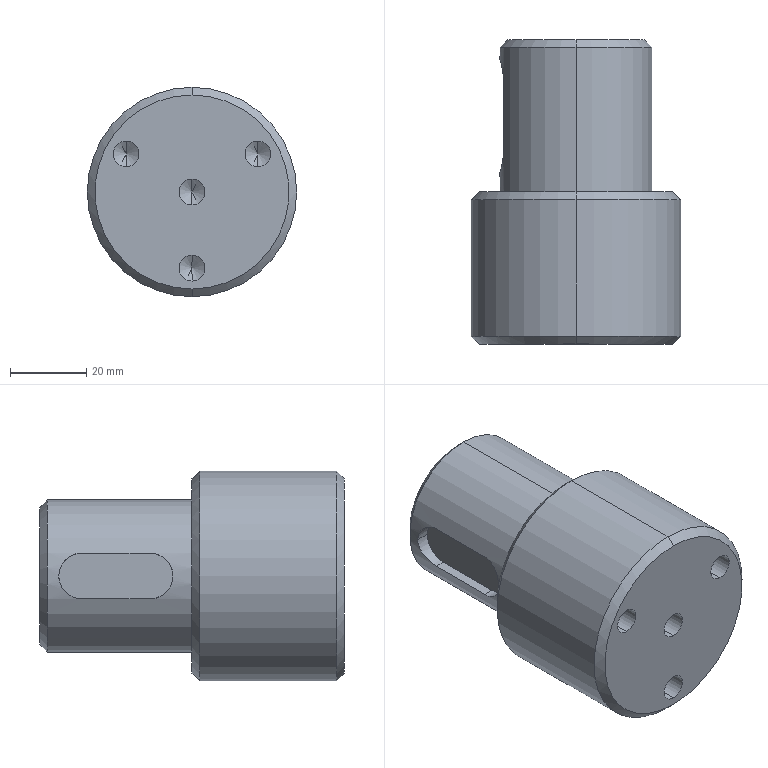Part | SolidWorks | features HoleWzd 2, Chamfer 1, Fillet 1, ICE 1, Revolution 1 | 1 solid | 40 faces | box 55 x 80 x 55 mm | volume 132055 mm3 | cylinder 18 | cone 16 | plane 6 | commonest cylinder face diameters 6.8 x8 12 x4 15.5 x2 40 x2 55 x2
STEP:
#1=CARTESIAN_POINT('',(0.,22.25,-16.6));
#2=VERTEX_POINT('',#1);
#3=CARTESIAN_POINT('',(0.,22.25,-23.4));
#4=VERTEX_POINT('',#3);
#5=CARTESIAN_POINT('',(0.,22.25,-20.));
#6=DIRECTION('',(0.,-1.,0.));
#7=DIRECTION('',(0.,0.,-1.));
#8=AXIS2_PLACEMENT_3D('',#5,#6,#7);
#9=CIRCLE('',#8,3.4);
#10=EDGE_CURVE('',#2,#4,#9,.T.);
#11=ORIENTED_EDGE('',*,*,#10,.F.);
#12=CARTESIAN_POINT('',(0.,0.,-16.6));
#13=VERTEX_POINT('',#12);
#14=CARTESIAN_POINT('',(0.,0.,-16.6));
#15=DIRECTION('',(0.,-1.,0.));
#16=VECTOR('',#15,1000.);
#17=LINE('',#14,#16);
#18=EDGE_CURVE('',#2,#13,#17,.T.);
#19=ORIENTED_EDGE('',*,*,#18,.T.);
#20=CARTESIAN_POINT('',(0.,0.,-23.4));
#21=VERTEX_POINT('',#20);
#22=CARTESIAN_POINT('',(0.,0.,-20.));
#23=DIRECTION('',(0.,-1.,0.));
#24=DIRECTION('',(0.,0.,-1.));
#25=AXIS2_PLACEMENT_3D('',#22,#23,#24);
#26=CIRCLE('',#25,3.4);
#27=EDGE_CURVE('',#13,#21,#26,.T.);
#28=ORIENTED_EDGE('',*,*,#27,.T.);
#29=CARTESIAN_POINT('',(0.,0.,-23.4));
#30=DIRECTION('',(0.,-1.,0.));
#31=VECTOR('',#30,1000.);
#32=LINE('',#29,#31);
#33=EDGE_CURVE('',#4,#21,#32,.T.);
#34=ORIENTED_EDGE('',*,*,#33,.F.);
#35=EDGE_LOOP('',(#11,#19,#28,#34));
#36=FACE_OUTER_BOUND('',#35,.T.);
#37=CARTESIAN_POINT('',(0.,0.,-20.));
#38=DIRECTION('',(0.,-1.,0.));
#39=DIRECTION('',(0.,0.,-1.));
#40=AXIS2_PLACEMENT_3D('',#37,#38,#39);
#41=CYLINDRICAL_SURFACE('',#40,3.4);
#42=ADVANCED_FACE('',(#36),#41,.F.);
#43=CARTESIAN_POINT('',(0.,24.293,-20.));
#44=VERTEX_POINT('',#43);
#45=CARTESIAN_POINT('',(0.,22.25,-23.4));
#46=DIRECTION('',(0.,-0.515,-0.8572));
#47=VECTOR('',#46,1000.);
#48=LINE('',#45,#47);
#49=EDGE_CURVE('',#44,#4,#48,.T.);
#50=ORIENTED_EDGE('',*,*,#49,.F.);
#51=CARTESIAN_POINT('',(0.,22.25,-16.6));
#52=DIRECTION('',(0.,-0.515,0.8572));
#53=VECTOR('',#52,1000.);
#54=LINE('',#51,#53);
#55=EDGE_CURVE('',#44,#2,#54,.T.);
#56=ORIENTED_EDGE('',*,*,#55,.T.);
#57=ORIENTED_EDGE('',*,*,#10,.T.);
#58=EDGE_LOOP('',(#50,#56,#57));
#59=FACE_OUTER_BOUND('',#58,.T.);
#60=CARTESIAN_POINT('',(0.,22.25,-20.));
#61=DIRECTION('',(0.,-1.,0.));
#62=DIRECTION('',(0.,0.,-1.));
#63=AXIS2_PLACEMENT_3D('',#60,#61,#62);
#64=CONICAL_SURFACE('',#63,3.4,1.03);
#65=ADVANCED_FACE('',(#59),#64,.F.);
#66=CARTESIAN_POINT('',(-17.321,22.25,13.4));
#67=VERTEX_POINT('',#66);
#68=CARTESIAN_POINT('',(-17.321,22.25,6.6));
#69=VERTEX_POINT('',#68);
#70=CARTESIAN_POINT('',(-17.321,22.25,10.));
#71=DIRECTION('',(0.,-1.,0.));
#72=DIRECTION('',(0.,0.,-1.));
#73=AXIS2_PLACEMENT_3D('',#70,#71,#72);
#74=CIRCLE('',#73,3.4);
#75=EDGE_CURVE('',#67,#69,#74,.T.);
#76=ORIENTED_EDGE('',*,*,#75,.F.);
#77=CARTESIAN_POINT('',(-17.321,0.,13.4));
#78=VERTEX_POINT('',#77);
#79=CARTESIAN_POINT('',(-17.321,0.,13.4));
#80=DIRECTION('',(0.,-1.,0.));
#81=VECTOR('',#80,1000.);
#82=LINE('',#79,#81);
#83=EDGE_CURVE('',#67,#78,#82,.T.);
#84=ORIENTED_EDGE('',*,*,#83,.T.);
#85=CARTESIAN_POINT('',(-17.321,0.,6.6));
#86=VERTEX_POINT('',#85);
#87=CARTESIAN_POINT('',(-17.321,0.,10.));
#88=DIRECTION('',(0.,-1.,0.));
#89=DIRECTION('',(0.,0.,-1.));
#90=AXIS2_PLACEMENT_3D('',#87,#88,#89);
#91=CIRCLE('',#90,3.4);
#92=EDGE_CURVE('',#78,#86,#91,.T.);
#93=ORIENTED_EDGE('',*,*,#92,.T.);
#94=CARTESIAN_POINT('',(-17.321,0.,6.6));
#95=DIRECTION('',(0.,-1.,0.));
#96=VECTOR('',#95,1000.);
#97=LINE('',#94,#96);
#98=EDGE_CURVE('',#69,#86,#97,.T.);
#99=ORIENTED_EDGE('',*,*,#98,.F.);
#100=EDGE_LOOP('',(#76,#84,#93,#99));
#101=FACE_OUTER_BOUND('',#100,.T.);
#102=CARTESIAN_POINT('',(-17.321,0.,10.));
#103=DIRECTION('',(0.,-1.,0.));
#104=DIRECTION('',(0.,0.,-1.));
#105=AXIS2_PLACEMENT_3D('',#102,#103,#104);
#106=CYLINDRICAL_SURFACE('',#105,3.4);
#107=ADVANCED_FACE('',(#101),#106,.F.);
#108=CARTESIAN_POINT('',(-17.321,24.293,10.));
#109=VERTEX_POINT('',#108);
#110=CARTESIAN_POINT('',(-17.321,22.25,6.6));
#111=DIRECTION('',(0.,-0.515,-0.8572));
#112=VECTOR('',#111,1000.);
#113=LINE('',#110,#112);
#114=EDGE_CURVE('',#109,#69,#113,.T.);
#115=ORIENTED_EDGE('',*,*,#114,.F.);
#116=CARTESIAN_POINT('',(-17.321,22.25,13.4));
#117=DIRECTION('',(0.,-0.515,0.8572));
#118=VECTOR('',#117,1000.);
#119=LINE('',#116,#118);
#120=EDGE_CURVE('',#109,#67,#119,.T.);
#121=ORIENTED_EDGE('',*,*,#120,.T.);
#122=ORIENTED_EDGE('',*,*,#75,.T.);
#123=EDGE_LOOP('',(#115,#121,#122));
#124=FACE_OUTER_BOUND('',#123,.T.);
#125=CARTESIAN_POINT('',(-17.321,22.25,10.));
#126=DIRECTION('',(0.,-1.,0.));
#127=DIRECTION('',(0.,0.,-1.));
#128=AXIS2_PLACEMENT_3D('',#125,#126,#127);
#129=CONICAL_SURFACE('',#128,3.4,1.03);
#130=ADVANCED_FACE('',(#124),#129,.F.);
#131=CARTESIAN_POINT('',(17.321,22.25,13.4));
#132=VERTEX_POINT('',#131);
#133=CARTESIAN_POINT('',(17.321,22.25,6.6));
#134=VERTEX_POINT('',#133);
#135=CARTESIAN_POINT('',(17.321,22.25,10.));
#136=DIRECTION('',(0.,-1.,0.));
#137=DIRECTION('',(0.,0.,-1.));
#138=AXIS2_PLACEMENT_3D('',#135,#136,#137);
#139=CIRCLE('',#138,3.4);
#140=EDGE_CURVE('',#132,#134,#139,.T.);
#141=ORIENTED_EDGE('',*,*,#140,.F.);
#142=CARTESIAN_POINT('',(17.321,0.,13.4));
#143=VERTEX_POINT('',#142);
#144=CARTESIAN_POINT('',(17.321,0.,13.4));
#145=DIRECTION('',(0.,-1.,0.));
#146=VECTOR('',#145,1000.);
#147=LINE('',#144,#146);
#148=EDGE_CURVE('',#132,#143,#147,.T.);
#149=ORIENTED_EDGE('',*,*,#148,.T.);
#150=CARTESIAN_POINT('',(17.321,0.,6.6));
#151=VERTEX_POINT('',#150);
#152=CARTESIAN_POINT('',(17.321,0.,10.));
#153=DIRECTION('',(0.,-1.,0.));
#154=DIRECTION('',(0.,0.,-1.));
#155=AXIS2_PLACEMENT_3D('',#152,#153,#154);
#156=CIRCLE('',#155,3.4);
#157=EDGE_CURVE('',#143,#151,#156,.T.);
#158=ORIENTED_EDGE('',*,*,#157,.T.);
#159=CARTESIAN_POINT('',(17.321,0.,6.6));
#160=DIRECTION('',(0.,-1.,0.));
#161=VECTOR('',#160,1000.);
#162=LINE('',#159,#161);
#163=EDGE_CURVE('',#134,#151,#162,.T.);
#164=ORIENTED_EDGE('',*,*,#163,.F.);
#165=EDGE_LOOP('',(#141,#149,#158,#164));
#166=FACE_OUTER_BOUND('',#165,.T.);
#167=CARTESIAN_POINT('',(17.321,0.,10.));
#168=DIRECTION('',(0.,-1.,0.));
#169=DIRECTION('',(0.,0.,-1.));
#170=AXIS2_PLACEMENT_3D('',#167,#168,#169);
#171=CYLINDRICAL_SURFACE('',#170,3.4);
#172=ADVANCED_FACE('',(#166),#171,.F.);
#173=CARTESIAN_POINT('',(17.321,24.293,10.));
#174=VERTEX_POINT('',#173);
#175=CARTESIAN_POINT('',(17.321,22.25,6.6));
#176=DIRECTION('',(0.,-0.515,-0.8572));
#177=VECTOR('',#176,1000.);
#178=LINE('',#175,#177);
#179=EDGE_CURVE('',#174,#134,#178,.T.);
#180=ORIENTED_EDGE('',*,*,#179,.F.);
#181=CARTESIAN_POINT('',(17.321,22.25,13.4));
#182=DIRECTION('',(0.,-0.515,0.8572));
#183=VECTOR('',#182,1000.);
#184=LINE('',#181,#183);
#185=EDGE_CURVE('',#174,#132,#184,.T.);
#186=ORIENTED_EDGE('',*,*,#185,.T.);
#187=ORIENTED_EDGE('',*,*,#140,.T.);
#188=EDGE_LOOP('',(#180,#186,#187));
#189=FACE_OUTER_BOUND('',#188,.T.);
#190=CARTESIAN_POINT('',(17.321,22.25,10.));
#191=DIRECTION('',(0.,-1.,0.));
#192=DIRECTION('',(0.,0.,-1.));
#193=AXIS2_PLACEMENT_3D('',#190,#191,#192);
#194=CONICAL_SURFACE('',#193,3.4,1.03);
#195=ADVANCED_FACE('',(#189),#194,.F.);
#196=CARTESIAN_POINT('',(0.,22.25,3.4));
#197=VERTEX_POINT('',#196);
#198=CARTESIAN_POINT('',(0.,22.25,-3.4));
#199=VERTEX_POINT('',#198);
#200=CARTESIAN_POINT('',(0.,22.25,0.));
#201=DIRECTION('',(0.,-1.,0.));
#202=DIRECTION('',(0.,0.,-1.));
#203=AXIS2_PLACEMENT_3D('',#200,#201,#202);
#204=CIRCLE('',#203,3.4);
#205=EDGE_CURVE('',#197,#199,#204,.T.);
#206=ORIENTED_EDGE('',*,*,#205,.F.);
#207=CARTESIAN_POINT('',(0.,0.,3.4));
#208=VERTEX_POINT('',#207);
#209=CARTESIAN_POINT('',(0.,0.,3.4));
#210=DIRECTION('',(0.,-1.,0.));
#211=VECTOR('',#210,1000.);
#212=LINE('',#209,#211);
#213=EDGE_CURVE('',#197,#208,#212,.T.);
#214=ORIENTED_EDGE('',*,*,#213,.T.);
#215=CARTESIAN_POINT('',(0.,0.,-3.4));
#216=VERTEX_POINT('',#215);
#217=CARTESIAN_POINT('',(0.,0.,0.));
#218=DIRECTION('',(0.,-1.,0.));
#219=DIRECTION('',(0.,0.,-1.));
#220=AXIS2_PLACEMENT_3D('',#217,#218,#219);
#221=CIRCLE('',#220,3.4);
#222=EDGE_CURVE('',#208,#216,#221,.T.);
#223=ORIENTED_EDGE('',*,*,#222,.T.);
#224=CARTESIAN_POINT('',(0.,0.,-3.4));
#225=DIRECTION('',(0.,-1.,0.));
#226=VECTOR('',#225,1000.);
#227=LINE('',#224,#226);
#228=EDGE_CURVE('',#199,#216,#227,.T.);
#229=ORIENTED_EDGE('',*,*,#228,.F.);
#230=EDGE_LOOP('',(#206,#214,#223,#229));
#231=FACE_OUTER_BOUND('',#230,.T.);
#232=CARTESIAN_POINT('',(0.,0.,0.));
#233=DIRECTION('',(0.,-1.,0.));
#234=DIRECTION('',(0.,0.,-1.));
#235=AXIS2_PLACEMENT_3D('',#232,#233,#234);
#236=CYLINDRICAL_SURFACE('',#235,3.4);
#237=ADVANCED_FACE('',(#231),#236,.F.);
#238=CARTESIAN_POINT('',(0.,24.293,0.));
#239=VERTEX_POINT('',#238);
#240=CARTESIAN_POINT('',(0.,22.25,-3.4));
#241=DIRECTION('',(0.,-0.515,-0.8572));
#242=VECTOR('',#241,1000.);
#243=LINE('',#240,#242);
#244=EDGE_CURVE('',#239,#199,#243,.T.);
#245=ORIENTED_EDGE('',*,*,#244,.F.);
#246=CARTESIAN_POINT('',(0.,22.25,3.4));
#247=DIRECTION('',(0.,-0.515,0.8572));
#248=VECTOR('',#247,1000.);
#249=LINE('',#246,#248);
#250=EDGE_CURVE('',#239,#197,#249,.T.);
#251=ORIENTED_EDGE('',*,*,#250,.T.);
#252=ORIENTED_EDGE('',*,*,#205,.T.);
#253=EDGE_LOOP('',(#245,#251,#252));
#254=FACE_OUTER_BOUND('',#253,.T.);
#255=CARTESIAN_POINT('',(0.,22.25,0.));
#256=DIRECTION('',(0.,-1.,0.));
#257=DIRECTION('',(0.,0.,-1.));
#258=AXIS2_PLACEMENT_3D('',#255,#256,#257);
#259=CONICAL_SURFACE('',#258,3.4,1.03);
#260=ADVANCED_FACE('',(#254),#259,.F.);
#261=CARTESIAN_POINT('',(0.,80.,18.));
#262=VERTEX_POINT('',#261);
#263=CARTESIAN_POINT('',(0.,80.,-18.));
#264=VERTEX_POINT('',#263);
#265=CARTESIAN_POINT('',(0.,80.,0.));
#266=DIRECTION('',(0.,1.,0.));
#267=DIRECTION('',(0.,0.,1.));
#268=AXIS2_PLACEMENT_3D('',#265,#266,#267);
#269=CIRCLE('',#268,18.);
#270=EDGE_CURVE('',#262,#264,#269,.T.);
#271=ORIENTED_EDGE('',*,*,#270,.F.);
#272=CARTESIAN_POINT('',(0.,78.,20.));
#273=VERTEX_POINT('',#272);
#274=CARTESIAN_POINT('',(0.,78.,20.));
#275=DIRECTION('',(0.,-0.7071,0.7071));
#276=VECTOR('',#275,1000.);
#277=LINE('',#274,#276);
#278=EDGE_CURVE('',#262,#273,#277,.T.);
#279=ORIENTED_EDGE('',*,*,#278,.T.);
#280=CARTESIAN_POINT('',(0.,78.,-20.));
#281=VERTEX_POINT('',#280);
#282=CARTESIAN_POINT('',(0.,78.,0.));
#283=DIRECTION('',(0.,-1.,0.));
#284=DIRECTION('',(0.,0.,1.));
#285=AXIS2_PLACEMENT_3D('',#282,#283,#284);
#286=CIRCLE('',#285,20.);
#287=EDGE_CURVE('',#281,#273,#286,.T.);
#288=ORIENTED_EDGE('',*,*,#287,.F.);
#289=CARTESIAN_POINT('',(0.,78.,-20.));
#290=DIRECTION('',(0.,-0.7071,-0.7071));
#291=VECTOR('',#290,1000.);
#292=LINE('',#289,#291);
#293=EDGE_CURVE('',#264,#281,#292,.T.);
#294=ORIENTED_EDGE('',*,*,#293,.F.);
#295=EDGE_LOOP('',(#271,#279,#288,#294));
#296=FACE_OUTER_BOUND('',#295,.T.);
#297=CARTESIAN_POINT('',(0.,78.,0.));
#298=DIRECTION('',(0.,-1.,0.));
#299=DIRECTION('',(0.,0.,-1.));
#300=AXIS2_PLACEMENT_3D('',#297,#298,#299);
#301=CONICAL_SURFACE('',#300,20.,0.7854);
#302=ADVANCED_FACE('',(#296),#301,.T.);
#303=CARTESIAN_POINT('',(0.,40.,25.5));
#304=VERTEX_POINT('',#303);
#305=CARTESIAN_POINT('',(0.,40.,-25.5));
#306=VERTEX_POINT('',#305);
#307=CARTESIAN_POINT('',(0.,40.,0.));
#308=DIRECTION('',(0.,1.,0.));
#309=DIRECTION('',(0.,0.,1.));
#310=AXIS2_PLACEMENT_3D('',#307,#308,#309);
#311=CIRCLE('',#310,25.5);
#312=EDGE_CURVE('',#304,#306,#311,.T.);
#313=ORIENTED_EDGE('',*,*,#312,.F.);
#314=CARTESIAN_POINT('',(0.,38.,27.5));
#315=VERTEX_POINT('',#314);
#316=CARTESIAN_POINT('',(0.,38.,27.5));
#317=DIRECTION('',(0.,-0.7071,0.7071));
#318=VECTOR('',#317,1000.);
#319=LINE('',#316,#318);
#320=EDGE_CURVE('',#304,#315,#319,.T.);
#321=ORIENTED_EDGE('',*,*,#320,.T.);
#322=CARTESIAN_POINT('',(0.,38.,-27.5));
#323=VERTEX_POINT('',#322);
#324=CARTESIAN_POINT('',(0.,38.,0.));
#325=DIRECTION('',(0.,-1.,0.));
#326=DIRECTION('',(0.,0.,1.));
#327=AXIS2_PLACEMENT_3D('',#324,#325,#326);
#328=CIRCLE('',#327,27.5);
#329=EDGE_CURVE('',#323,#315,#328,.T.);
#330=ORIENTED_EDGE('',*,*,#329,.F.);
#331=CARTESIAN_POINT('',(0.,38.,-27.5));
#332=DIRECTION('',(0.,-0.7071,-0.7071));
#333=VECTOR('',#332,1000.);
#334=LINE('',#331,#333);
#335=EDGE_CURVE('',#306,#323,#334,.T.);
#336=ORIENTED_EDGE('',*,*,#335,.F.);
#337=EDGE_LOOP('',(#313,#321,#330,#336));
#338=FACE_OUTER_BOUND('',#337,.T.);
#339=CARTESIAN_POINT('',(0.,38.,0.));
#340=DIRECTION('',(0.,-1.,0.));
#341=DIRECTION('',(0.,0.,-1.));
#342=AXIS2_PLACEMENT_3D('',#339,#340,#341);
#343=CONICAL_SURFACE('',#342,27.5,0.7854);
#344=ADVANCED_FACE('',(#338),#343,.T.);
#345=CARTESIAN_POINT('',(0.,0.,-25.5));
#346=VERTEX_POINT('',#345);
#347=CARTESIAN_POINT('',(0.,0.,25.5));
#348=VERTEX_POINT('',#347);
#349=CARTESIAN_POINT('',(0.,0.,0.));
#350=DIRECTION('',(0.,-1.,0.));
#351=DIRECTION('',(0.,0.,-1.));
#352=AXIS2_PLACEMENT_3D('',#349,#350,#351);
#353=CIRCLE('',#352,25.5);
#354=EDGE_CURVE('',#346,#348,#353,.T.);
#355=ORIENTED_EDGE('',*,*,#354,.F.);
#356=CARTESIAN_POINT('',(0.,2.,-27.5));
#357=VERTEX_POINT('',#356);
#358=CARTESIAN_POINT('',(0.,0.,-25.5));
#359=DIRECTION('',(0.,0.7071,-0.7071));
#360=VECTOR('',#359,1000.);
#361=LINE('',#358,#360);
#362=EDGE_CURVE('',#346,#357,#361,.T.);
#363=ORIENTED_EDGE('',*,*,#362,.T.);
#364=CARTESIAN_POINT('',(0.,2.,27.5));
#365=VERTEX_POINT('',#364);
#366=CARTESIAN_POINT('',(0.,2.,0.));
#367=DIRECTION('',(0.,1.,0.));
#368=DIRECTION('',(0.,0.,-1.));
#369=AXIS2_PLACEMENT_3D('',#366,#367,#368);
#370=CIRCLE('',#369,27.5);
#371=EDGE_CURVE('',#365,#357,#370,.T.);
#372=ORIENTED_EDGE('',*,*,#371,.F.);
#373=CARTESIAN_POINT('',(0.,0.,25.5));
#374=DIRECTION('',(0.,0.7071,0.7071));
#375=VECTOR('',#374,1000.);
#376=LINE('',#373,#375);
#377=EDGE_CURVE('',#348,#365,#376,.T.);
#378=ORIENTED_EDGE('',*,*,#377,.F.);
#379=EDGE_LOOP('',(#355,#363,#372,#378));
#380=FACE_OUTER_BOUND('',#379,.T.);
#381=CARTESIAN_POINT('',(0.,0.,0.));
#382=DIRECTION('',(0.,1.,0.));
#383=DIRECTION('',(0.,0.,1.));
#384=AXIS2_PLACEMENT_3D('',#381,#382,#383);
#385=CONICAL_SURFACE('',#384,25.5,0.7854);
#386=ADVANCED_FACE('',(#380),#385,.T.);
#387=CARTESIAN_POINT('',(0.,39.5,-7.75));
#388=VERTEX_POINT('',#387);
#389=CARTESIAN_POINT('',(0.,39.5,7.75));
#390=VERTEX_POINT('',#389);
#391=CARTESIAN_POINT('',(0.,39.5,0.));
#392=DIRECTION('',(0.,1.,0.));
#393=DIRECTION('',(0.,0.,1.));
#394=AXIS2_PLACEMENT_3D('',#391,#392,#393);
#395=CIRCLE('',#394,7.75);
#396=EDGE_CURVE('',#388,#390,#395,.T.);
#397=ORIENTED_EDGE('',*,*,#396,.F.);
#398=CARTESIAN_POINT('',(0.,80.,-7.75));
#399=VERTEX_POINT('',#398);
#400=CARTESIAN_POINT('',(0.,80.,-7.75));
#401=DIRECTION('',(0.,1.,0.));
#402=VECTOR('',#401,1000.);
#403=LINE('',#400,#402);
#404=EDGE_CURVE('',#388,#399,#403,.T.);
#405=ORIENTED_EDGE('',*,*,#404,.T.);
#406=CARTESIAN_POINT('',(0.,80.,7.75));
#407=VERTEX_POINT('',#406);
#408=CARTESIAN_POINT('',(0.,80.,0.));
#409=DIRECTION('',(0.,1.,0.));
#410=DIRECTION('',(0.,0.,1.));
#411=AXIS2_PLACEMENT_3D('',#408,#409,#410);
#412=CIRCLE('',#411,7.75);
#413=EDGE_CURVE('',#399,#407,#412,.T.);
#414=ORIENTED_EDGE('',*,*,#413,.T.);
#415=CARTESIAN_POINT('',(0.,80.,7.75));
#416=DIRECTION('',(0.,1.,0.));
#417=VECTOR('',#416,1000.);
#418=LINE('',#415,#417);
#419=EDGE_CURVE('',#390,#407,#418,.T.);
#420=ORIENTED_EDGE('',*,*,#419,.F.);
#421=EDGE_LOOP('',(#397,#405,#414,#420));
#422=FACE_OUTER_BOUND('',#421,.T.);
#423=CARTESIAN_POINT('',(0.,80.,0.));
#424=DIRECTION('',(0.,1.,0.));
#425=DIRECTION('',(0.,0.,1.));
#426=AXIS2_PLACEMENT_3D('',#423,#424,#425);
#427=CYLINDRICAL_SURFACE('',#426,7.75);
#428=ADVANCED_FACE('',(#422),#427,.F.);
#429=CARTESIAN_POINT('',(0.,34.843,0.));
#430=VERTEX_POINT('',#429);
#431=CARTESIAN_POINT('',(0.,39.5,7.75));
#432=DIRECTION('',(0.,0.515,0.8572));
#433=VECTOR('',#432,1000.);
#434=LINE('',#431,#433);
#435=EDGE_CURVE('',#430,#390,#434,.T.);
#436=ORIENTED_EDGE('',*,*,#435,.F.);
#437=CARTESIAN_POINT('',(0.,39.5,-7.75));
#438=DIRECTION('',(0.,0.515,-0.8572));
#439=VECTOR('',#438,1000.);
#440=LINE('',#437,#439);
#441=EDGE_CURVE('',#430,#388,#440,.T.);
#442=ORIENTED_EDGE('',*,*,#441,.T.);
#443=ORIENTED_EDGE('',*,*,#396,.T.);
#444=EDGE_LOOP('',(#436,#442,#443));
#445=FACE_OUTER_BOUND('',#444,.T.);
#446=CARTESIAN_POINT('',(0.,39.5,0.));
#447=DIRECTION('',(0.,1.,0.));
#448=DIRECTION('',(0.,0.,1.));
#449=AXIS2_PLACEMENT_3D('',#446,#447,#448);
#450=CONICAL_SURFACE('',#449,7.75,1.03);
#451=ADVANCED_FACE('',(#445),#450,.F.);
#452=ORIENTED_EDGE('',*,*,#329,.T.);
#453=CARTESIAN_POINT('',(0.,0.,27.5));
#454=DIRECTION('',(0.,-1.,0.));
#455=VECTOR('',#454,1000.);
#456=LINE('',#453,#455);
#457=EDGE_CURVE('',#315,#365,#456,.T.);
#458=ORIENTED_EDGE('',*,*,#457,.T.);
#459=ORIENTED_EDGE('',*,*,#371,.T.);
#460=CARTESIAN_POINT('',(0.,0.,-27.5));
#461=DIRECTION('',(0.,-1.,0.));
#462=VECTOR('',#461,1000.);
#463=LINE('',#460,#462);
#464=EDGE_CURVE('',#323,#357,#463,.T.);
#465=ORIENTED_EDGE('',*,*,#464,.F.);
#466=EDGE_LOOP('',(#452,#458,#459,#465));
#467=FACE_OUTER_BOUND('',#466,.T.);
#468=CARTESIAN_POINT('',(0.,0.,0.));
#469=DIRECTION('',(0.,-1.,0.));
#470=DIRECTION('',(0.,0.,-1.));
#471=AXIS2_PLACEMENT_3D('',#468,#469,#470);
#472=CYLINDRICAL_SURFACE('',#471,27.5);
#473=ADVANCED_FACE('',(#467),#472,.T.);
#474=ORIENTED_EDGE('',*,*,#287,.T.);
#475=CARTESIAN_POINT('',(0.,40.,20.));
#476=VERTEX_POINT('',#475);
#477=CARTESIAN_POINT('',(0.,0.,20.));
#478=DIRECTION('',(0.,-1.,0.));
#479=VECTOR('',#478,1000.);
#480=LINE('',#477,#479);
#481=EDGE_CURVE('',#273,#476,#480,.T.);
#482=ORIENTED_EDGE('',*,*,#481,.T.);
#483=CARTESIAN_POINT('',(0.,40.,-20.));
#484=VERTEX_POINT('',#483);
#485=CARTESIAN_POINT('',(0.,40.,0.));
#486=DIRECTION('',(0.,-1.,0.));
#487=DIRECTION('',(0.,0.,-1.));
#488=AXIS2_PLACEMENT_3D('',#485,#486,#487);
#489=CIRCLE('',#488,20.);
#490=EDGE_CURVE('',#484,#476,#489,.T.);
#491=ORIENTED_EDGE('',*,*,#490,.F.);
#492=CARTESIAN_POINT('',(0.,0.,-20.));
#493=DIRECTION('',(0.,-1.,0.));
#494=VECTOR('',#493,1000.);
#495=LINE('',#492,#494);
#496=EDGE_CURVE('',#281,#484,#495,.T.);
#497=ORIENTED_EDGE('',*,*,#496,.F.);
#498=EDGE_LOOP('',(#474,#482,#491,#497));
#499=FACE_OUTER_BOUND('',#498,.T.);
#500=CARTESIAN_POINT('',(0.,0.,0.));
#501=DIRECTION('',(0.,-1.,0.));
#502=DIRECTION('',(0.,0.,-1.));
#503=AXIS2_PLACEMENT_3D('',#500,#501,#502);
#504=CYLINDRICAL_SURFACE('',#503,20.);
#505=ADVANCED_FACE('',(#499),#504,.T.);
#506=CARTESIAN_POINT('',(0.,0.,-20.));
#507=DIRECTION('',(0.,-1.,0.));
#508=DIRECTION('',(0.,0.,-1.));
#509=AXIS2_PLACEMENT_3D('',#506,#507,#508);
#510=CIRCLE('',#509,3.4);
#511=EDGE_CURVE('',#21,#13,#510,.T.);
#512=ORIENTED_EDGE('',*,*,#511,.F.);
#513=ORIENTED_EDGE('',*,*,#27,.F.);
#514=EDGE_LOOP('',(#512,#513));
#515=FACE_BOUND('',#514,.T.);
#516=CARTESIAN_POINT('',(-17.321,0.,10.));
#517=DIRECTION('',(0.,-1.,0.));
#518=DIRECTION('',(0.,0.,-1.));
#519=AXIS2_PLACEMENT_3D('',#516,#517,#518);
#520=CIRCLE('',#519,3.4);
#521=EDGE_CURVE('',#86,#78,#520,.T.);
#522=ORIENTED_EDGE('',*,*,#521,.F.);
#523=ORIENTED_EDGE('',*,*,#92,.F.);
#524=EDGE_LOOP('',(#522,#523));
#525=FACE_BOUND('',#524,.T.);
#526=CARTESIAN_POINT('',(17.321,0.,10.));
#527=DIRECTION('',(0.,-1.,0.));
#528=DIRECTION('',(0.,0.,-1.));
#529=AXIS2_PLACEMENT_3D('',#526,#527,#528);
#530=CIRCLE('',#529,3.4);
#531=EDGE_CURVE('',#151,#143,#530,.T.);
#532=ORIENTED_EDGE('',*,*,#531,.F.);
#533=ORIENTED_EDGE('',*,*,#157,.F.);
#534=EDGE_LOOP('',(#532,#533));
#535=FACE_BOUND('',#534,.T.);
#536=CARTESIAN_POINT('',(0.,0.,0.));
#537=DIRECTION('',(0.,-1.,0.));
#538=DIRECTION('',(0.,0.,-1.));
#539=AXIS2_PLACEMENT_3D('',#536,#537,#538);
#540=CIRCLE('',#539,3.4);
#541=EDGE_CURVE('',#216,#208,#540,.T.);
#542=ORIENTED_EDGE('',*,*,#541,.F.);
#543=ORIENTED_EDGE('',*,*,#222,.F.);
#544=EDGE_LOOP('',(#542,#543));
#545=FACE_BOUND('',#544,.T.);
#546=CARTESIAN_POINT('',(0.,0.,0.));
#547=DIRECTION('',(0.,-1.,0.));
#548=DIRECTION('',(0.,0.,-1.));
#549=AXIS2_PLACEMENT_3D('',#546,#547,#548);
#550=CIRCLE('',#549,25.5);
#551=EDGE_CURVE('',#348,#346,#550,.T.);
#552=ORIENTED_EDGE('',*,*,#551,.T.);
#553=ORIENTED_EDGE('',*,*,#354,.T.);
#554=EDGE_LOOP('',(#552,#553));
#555=FACE_OUTER_BOUND('',#554,.T.);
#556=CARTESIAN_POINT('',(27.5,0.,0.));
#557=DIRECTION('',(0.,-1.,0.));
#558=DIRECTION('',(0.,0.,-1.));
#559=AXIS2_PLACEMENT_3D('',#556,#557,#558);
#560=PLANE('',#559);
#561=ADVANCED_FACE('',(#515,#525,#535,#545,#555),#560,.T.);
#562=CARTESIAN_POINT('',(0.,80.,0.));
#563=DIRECTION('',(0.,1.,0.));
#564=DIRECTION('',(0.,0.,1.));
#565=AXIS2_PLACEMENT_3D('',#562,#563,#564);
#566=CIRCLE('',#565,18.);
#567=EDGE_CURVE('',#264,#262,#566,.T.);
#568=ORIENTED_EDGE('',*,*,#567,.T.);
#569=ORIENTED_EDGE('',*,*,#270,.T.);
#570=EDGE_LOOP('',(#568,#569));
#571=FACE_OUTER_BOUND('',#570,.T.);
#572=CARTESIAN_POINT('',(0.,80.,0.));
#573=DIRECTION('',(0.,1.,0.));
#574=DIRECTION('',(0.,0.,1.));
#575=AXIS2_PLACEMENT_3D('',#572,#573,#574);
#576=CIRCLE('',#575,7.75);
#577=EDGE_CURVE('',#407,#399,#576,.T.);
#578=ORIENTED_EDGE('',*,*,#577,.F.);
#579=ORIENTED_EDGE('',*,*,#413,.F.);
#580=EDGE_LOOP('',(#578,#579));
#581=FACE_BOUND('',#580,.T.);
#582=CARTESIAN_POINT('',(0.,80.,0.));
#583=DIRECTION('',(0.,1.,0.));
#584=DIRECTION('',(0.,0.,1.));
#585=AXIS2_PLACEMENT_3D('',#582,#583,#584);
#586=PLANE('',#585);
#587=ADVANCED_FACE('',(#571,#581),#586,.T.);
#588=ORIENTED_EDGE('',*,*,#481,.F.);
#589=CARTESIAN_POINT('',(0.,78.,0.));
#590=DIRECTION('',(0.,-1.,0.));
#591=DIRECTION('',(0.,0.,1.));
#592=AXIS2_PLACEMENT_3D('',#589,#590,#591);
#593=CIRCLE('',#592,20.);
#594=EDGE_CURVE('',#273,#281,#593,.T.);
#595=ORIENTED_EDGE('',*,*,#594,.T.);
#596=ORIENTED_EDGE('',*,*,#496,.T.);
#597=CARTESIAN_POINT('',(0.,40.,0.));
#598=DIRECTION('',(0.,-1.,0.));
#599=DIRECTION('',(0.,0.,-1.));
#600=AXIS2_PLACEMENT_3D('',#597,#598,#599);
#601=CIRCLE('',#600,20.);
#602=EDGE_CURVE('',#476,#484,#601,.T.);
#603=ORIENTED_EDGE('',*,*,#602,.F.);
#604=EDGE_LOOP('',(#588,#595,#596,#603));
#605=FACE_OUTER_BOUND('',#604,.T.);
#606=CARTESIAN_POINT('',(-19.079,51.,6.));
#607=VERTEX_POINT('',#606);
#608=CARTESIAN_POINT('',(-19.079,69.,6.));
#609=VERTEX_POINT('',#608);
#610=CARTESIAN_POINT('',(-19.079,0.,6.));
#611=DIRECTION('',(0.,1.,0.));
#612=VECTOR('',#611,1000.);
#613=LINE('',#610,#612);
#614=EDGE_CURVE('',#607,#609,#613,.T.);
#615=ORIENTED_EDGE('',*,*,#614,.F.);
#616=CARTESIAN_POINT('',(-20.,45.,0.));
#617=VERTEX_POINT('',#616);
#618=CARTESIAN_POINT('',(-19.079,51.,6.));
#619=CARTESIAN_POINT('',(-19.079,50.601,6.));
#620=CARTESIAN_POINT('',(-19.091,50.21,5.961));
#621=CARTESIAN_POINT('',(-19.127,49.633,5.845));
#622=CARTESIAN_POINT('',(-19.141,49.442,5.798));
#623=CARTESIAN_POINT('',(-19.176,49.064,5.683));
#624=CARTESIAN_POINT('',(-19.196,48.877,5.615));
#625=CARTESIAN_POINT('',(-19.261,48.333,5.389));
#626=CARTESIAN_POINT('',(-19.312,47.99,5.205));
#627=CARTESIAN_POINT('',(-19.396,47.502,4.879));
#628=CARTESIAN_POINT('',(-19.425,47.343,4.761));
#629=CARTESIAN_POINT('',(-19.485,47.04,4.512));
#630=CARTESIAN_POINT('',(-19.515,46.896,4.381));
#631=CARTESIAN_POINT('',(-19.604,46.484,3.969));
#632=CARTESIAN_POINT('',(-19.663,46.236,3.669));
#633=CARTESIAN_POINT('',(-19.774,45.797,3.014));
#634=CARTESIAN_POINT('',(-19.824,45.612,2.669));
#635=CARTESIAN_POINT('',(-19.887,45.387,2.129));
#636=CARTESIAN_POINT('',(-19.906,45.32,1.945));
#637=CARTESIAN_POINT('',(-19.939,45.205,1.568));
#638=CARTESIAN_POINT('',(-19.954,45.156,1.375));
#639=CARTESIAN_POINT('',(-19.988,45.039,0.7921));
#640=CARTESIAN_POINT('',(-20.,45.,0.3986));
#641=CARTESIAN_POINT('',(-20.,45.,0.));
#642=B_SPLINE_CURVE_WITH_KNOTS('',3,(#618,#619,#620,#621,#622,#623,#624,#625,#626,#627,#628,#629,#630,#631,#632,#633,#634,#635,#636,#637,#638,#639,#640,#641),.UNSPECIFIED.,.F.,.F.,(4,2,2,2,2,2,2,2,2,2,2,4),(0.,0.001178,0.001768,0.002357,0.003535,0.004125,0.004714,0.005892,0.007071,0.00766,0.008249,0.009428),.UNSPECIFIED.);
#643=EDGE_CURVE('',#607,#617,#642,.T.);
#644=ORIENTED_EDGE('',*,*,#643,.T.);
#645=CARTESIAN_POINT('',(-19.079,51.,-6.));
#646=VERTEX_POINT('',#645);
#647=CARTESIAN_POINT('',(-20.,45.,0.));
#648=CARTESIAN_POINT('',(-20.,45.,-0.3986));
#649=CARTESIAN_POINT('',(-19.988,45.039,-0.7902));
#650=CARTESIAN_POINT('',(-19.954,45.155,-1.367));
#651=CARTESIAN_POINT('',(-19.94,45.202,-1.558));
#652=CARTESIAN_POINT('',(-19.907,45.318,-1.936));
#653=CARTESIAN_POINT('',(-19.888,45.385,-2.123));
#654=CARTESIAN_POINT('',(-19.825,45.611,-2.667));
#655=CARTESIAN_POINT('',(-19.775,45.795,-3.011));
#656=CARTESIAN_POINT('',(-19.692,46.122,-3.499));
#657=CARTESIAN_POINT('',(-19.663,46.239,-3.657));
#658=CARTESIAN_POINT('',(-19.605,46.488,-3.96));
#659=CARTESIAN_POINT('',(-19.575,46.619,-4.105));
#660=CARTESIAN_POINT('',(-19.485,47.032,-4.517));
#661=CARTESIAN_POINT('',(-19.426,47.332,-4.764));
#662=CARTESIAN_POINT('',(-19.313,47.986,-5.203));
#663=CARTESIAN_POINT('',(-19.261,48.331,-5.388));
#664=CARTESIAN_POINT('',(-19.196,48.872,-5.613));
#665=CARTESIAN_POINT('',(-19.177,49.056,-5.68));
#666=CARTESIAN_POINT('',(-19.142,49.432,-5.795));
#667=CARTESIAN_POINT('',(-19.127,49.625,-5.844));
#668=CARTESIAN_POINT('',(-19.091,50.208,-5.961));
#669=CARTESIAN_POINT('',(-19.079,50.601,-6.));
#670=CARTESIAN_POINT('',(-19.079,51.,-6.));
#671=B_SPLINE_CURVE_WITH_KNOTS('',3,(#647,#648,#649,#650,#651,#652,#653,#654,#655,#656,#657,#658,#659,#660,#661,#662,#663,#664,#665,#666,#667,#668,#669,#670),.UNSPECIFIED.,.F.,.F.,(4,2,2,2,2,2,2,2,2,2,2,4),(0.,0.001178,0.001768,0.002357,0.003535,0.004125,0.004714,0.005892,0.007071,0.00766,0.008249,0.009428),.UNSPECIFIED.);
#672=EDGE_CURVE('',#617,#646,#671,.T.);
#673=ORIENTED_EDGE('',*,*,#672,.T.);
#674=CARTESIAN_POINT('',(-19.079,69.,-6.));
#675=VERTEX_POINT('',#674);
#676=CARTESIAN_POINT('',(-19.079,0.,-6.));
#677=DIRECTION('',(0.,-1.,0.));
#678=VECTOR('',#677,1000.);
#679=LINE('',#676,#678);
#680=EDGE_CURVE('',#675,#646,#679,.T.);
#681=ORIENTED_EDGE('',*,*,#680,.F.);
#682=CARTESIAN_POINT('',(-20.,75.,0.));
#683=VERTEX_POINT('',#682);
#684=CARTESIAN_POINT('',(-19.079,69.,-6.));
#685=CARTESIAN_POINT('',(-19.079,69.399,-6.));
#686=CARTESIAN_POINT('',(-19.091,69.79,-5.961));
#687=CARTESIAN_POINT('',(-19.127,70.367,-5.845));
#688=CARTESIAN_POINT('',(-19.141,70.558,-5.798));
#689=CARTESIAN_POINT('',(-19.176,70.936,-5.683));
#690=CARTESIAN_POINT('',(-19.196,71.123,-5.615));
#691=CARTESIAN_POINT('',(-19.261,71.667,-5.389));
#692=CARTESIAN_POINT('',(-19.312,72.01,-5.205));
#693=CARTESIAN_POINT('',(-19.396,72.498,-4.879));
#694=CARTESIAN_POINT('',(-19.425,72.657,-4.761));
#695=CARTESIAN_POINT('',(-19.485,72.96,-4.512));
#696=CARTESIAN_POINT('',(-19.515,73.104,-4.381));
#697=CARTESIAN_POINT('',(-19.604,73.516,-3.969));
#698=CARTESIAN_POINT('',(-19.663,73.764,-3.669));
#699=CARTESIAN_POINT('',(-19.774,74.203,-3.014));
#700=CARTESIAN_POINT('',(-19.824,74.388,-2.669));
#701=CARTESIAN_POINT('',(-19.887,74.613,-2.129));
#702=CARTESIAN_POINT('',(-19.906,74.68,-1.945));
#703=CARTESIAN_POINT('',(-19.939,74.795,-1.568));
#704=CARTESIAN_POINT('',(-19.954,74.844,-1.375));
#705=CARTESIAN_POINT('',(-19.988,74.961,-0.7921));
#706=CARTESIAN_POINT('',(-20.,75.,-0.3986));
#707=CARTESIAN_POINT('',(-20.,75.,0.));
#708=B_SPLINE_CURVE_WITH_KNOTS('',3,(#684,#685,#686,#687,#688,#689,#690,#691,#692,#693,#694,#695,#696,#697,#698,#699,#700,#701,#702,#703,#704,#705,#706,#707),.UNSPECIFIED.,.F.,.F.,(4,2,2,2,2,2,2,2,2,2,2,4),(0.,0.001178,0.001768,0.002357,0.003535,0.004125,0.004714,0.005892,0.007071,0.00766,0.008249,0.009428),.UNSPECIFIED.);
#709=EDGE_CURVE('',#675,#683,#708,.T.);
#710=ORIENTED_EDGE('',*,*,#709,.T.);
#711=CARTESIAN_POINT('',(-20.,75.,0.));
#712=CARTESIAN_POINT('',(-20.,75.,0.3986));
#713=CARTESIAN_POINT('',(-19.988,74.961,0.7902));
#714=CARTESIAN_POINT('',(-19.954,74.845,1.367));
#715=CARTESIAN_POINT('',(-19.94,74.798,1.558));
#716=CARTESIAN_POINT('',(-19.907,74.682,1.936));
#717=CARTESIAN_POINT('',(-19.888,74.615,2.123));
#718=CARTESIAN_POINT('',(-19.825,74.389,2.667));
#719=CARTESIAN_POINT('',(-19.775,74.205,3.011));
#720=CARTESIAN_POINT('',(-19.692,73.878,3.499));
#721=CARTESIAN_POINT('',(-19.663,73.761,3.657));
#722=CARTESIAN_POINT('',(-19.605,73.512,3.96));
#723=CARTESIAN_POINT('',(-19.575,73.381,4.105));
#724=CARTESIAN_POINT('',(-19.485,72.968,4.517));
#725=CARTESIAN_POINT('',(-19.426,72.668,4.764));
#726=CARTESIAN_POINT('',(-19.313,72.014,5.203));
#727=CARTESIAN_POINT('',(-19.261,71.669,5.388));
#728=CARTESIAN_POINT('',(-19.196,71.128,5.613));
#729=CARTESIAN_POINT('',(-19.177,70.944,5.68));
#730=CARTESIAN_POINT('',(-19.142,70.568,5.795));
#731=CARTESIAN_POINT('',(-19.127,70.375,5.844));
#732=CARTESIAN_POINT('',(-19.091,69.792,5.961));
#733=CARTESIAN_POINT('',(-19.079,69.399,6.));
#734=CARTESIAN_POINT('',(-19.079,69.,6.));
#735=B_SPLINE_CURVE_WITH_KNOTS('',3,(#711,#712,#713,#714,#715,#716,#717,#718,#719,#720,#721,#722,#723,#724,#725,#726,#727,#728,#729,#730,#731,#732,#733,#734),.UNSPECIFIED.,.F.,.F.,(4,2,2,2,2,2,2,2,2,2,2,4),(0.,0.001178,0.001768,0.002357,0.003535,0.004125,0.004714,0.005892,0.007071,0.00766,0.008249,0.009428),.UNSPECIFIED.);
#736=EDGE_CURVE('',#683,#609,#735,.T.);
#737=ORIENTED_EDGE('',*,*,#736,.T.);
#738=EDGE_LOOP('',(#615,#644,#673,#681,#710,#737));
#739=FACE_BOUND('',#738,.T.);
#740=CARTESIAN_POINT('',(0.,0.,0.));
#741=DIRECTION('',(0.,-1.,0.));
#742=DIRECTION('',(0.,0.,-1.));
#743=AXIS2_PLACEMENT_3D('',#740,#741,#742);
#744=CYLINDRICAL_SURFACE('',#743,20.);
#745=ADVANCED_FACE('',(#605,#739),#744,.T.);
#746=CARTESIAN_POINT('',(0.,40.,0.));
#747=DIRECTION('',(0.,1.,0.));
#748=DIRECTION('',(0.,0.,1.));
#749=AXIS2_PLACEMENT_3D('',#746,#747,#748);
#750=CIRCLE('',#749,25.5);
#751=EDGE_CURVE('',#306,#304,#750,.T.);
#752=ORIENTED_EDGE('',*,*,#751,.T.);
#753=ORIENTED_EDGE('',*,*,#312,.T.);
#754=EDGE_LOOP('',(#752,#753));
#755=FACE_OUTER_BOUND('',#754,.T.);
#756=ORIENTED_EDGE('',*,*,#490,.T.);
#757=ORIENTED_EDGE('',*,*,#602,.T.);
#758=EDGE_LOOP('',(#756,#757));
#759=FACE_BOUND('',#758,.T.);
#760=CARTESIAN_POINT('',(20.,40.,0.));
#761=DIRECTION('',(0.,1.,0.));
#762=DIRECTION('',(0.,0.,1.));
#763=AXIS2_PLACEMENT_3D('',#760,#761,#762);
#764=PLANE('',#763);
#765=ADVANCED_FACE('',(#755,#759),#764,.T.);
#766=ORIENTED_EDGE('',*,*,#457,.F.);
#767=CARTESIAN_POINT('',(0.,38.,0.));
#768=DIRECTION('',(0.,-1.,0.));
#769=DIRECTION('',(0.,0.,1.));
#770=AXIS2_PLACEMENT_3D('',#767,#768,#769);
#771=CIRCLE('',#770,27.5);
#772=EDGE_CURVE('',#315,#323,#771,.T.);
#773=ORIENTED_EDGE('',*,*,#772,.T.);
#774=ORIENTED_EDGE('',*,*,#464,.T.);
#775=CARTESIAN_POINT('',(0.,2.,0.));
#776=DIRECTION('',(0.,1.,0.));
#777=DIRECTION('',(0.,0.,-1.));
#778=AXIS2_PLACEMENT_3D('',#775,#776,#777);
#779=CIRCLE('',#778,27.5);
#780=EDGE_CURVE('',#357,#365,#779,.T.);
#781=ORIENTED_EDGE('',*,*,#780,.T.);
#782=EDGE_LOOP('',(#766,#773,#774,#781));
#783=FACE_OUTER_BOUND('',#782,.T.);
#784=CARTESIAN_POINT('',(0.,0.,0.));
#785=DIRECTION('',(0.,-1.,0.));
#786=DIRECTION('',(0.,0.,-1.));
#787=AXIS2_PLACEMENT_3D('',#784,#785,#786);
#788=CYLINDRICAL_SURFACE('',#787,27.5);
#789=ADVANCED_FACE('',(#783),#788,.T.);
#790=CARTESIAN_POINT('',(-16.5,69.,6.));
#791=VERTEX_POINT('',#790);
#792=CARTESIAN_POINT('',(-16.5,51.,6.));
#793=VERTEX_POINT('',#792);
#794=CARTESIAN_POINT('',(-16.5,75.,6.));
#795=DIRECTION('',(0.,-1.,0.));
#796=VECTOR('',#795,1000.);
#797=LINE('',#794,#796);
#798=EDGE_CURVE('',#791,#793,#797,.T.);
#799=ORIENTED_EDGE('',*,*,#798,.T.);
#800=CARTESIAN_POINT('',(-19.079,51.,6.));
#801=DIRECTION('',(-1.,0.,0.));
#802=VECTOR('',#801,1000.);
#803=LINE('',#800,#802);
#804=EDGE_CURVE('',#793,#607,#803,.T.);
#805=ORIENTED_EDGE('',*,*,#804,.T.);
#806=ORIENTED_EDGE('',*,*,#614,.T.);
#807=CARTESIAN_POINT('',(-16.5,69.,6.));
#808=DIRECTION('',(1.,0.,0.));
#809=VECTOR('',#808,1000.);
#810=LINE('',#807,#809);
#811=EDGE_CURVE('',#609,#791,#810,.T.);
#812=ORIENTED_EDGE('',*,*,#811,.T.);
#813=EDGE_LOOP('',(#799,#805,#806,#812));
#814=FACE_OUTER_BOUND('',#813,.T.);
#815=CARTESIAN_POINT('',(-27.5,75.,6.));
#816=DIRECTION('',(0.,0.,1.));
#817=DIRECTION('',(0.,-1.,0.));
#818=AXIS2_PLACEMENT_3D('',#815,#816,#817);
#819=PLANE('',#818);
#820=ADVANCED_FACE('',(#814),#819,.F.);
#821=ORIENTED_EDGE('',*,*,#680,.T.);
#822=CARTESIAN_POINT('',(-16.5,51.,-6.));
#823=VERTEX_POINT('',#822);
#824=CARTESIAN_POINT('',(-16.5,51.,-6.));
#825=DIRECTION('',(1.,0.,0.));
#826=VECTOR('',#825,1000.);
#827=LINE('',#824,#826);
#828=EDGE_CURVE('',#646,#823,#827,.T.);
#829=ORIENTED_EDGE('',*,*,#828,.T.);
#830=CARTESIAN_POINT('',(-16.5,69.,-6.));
#831=VERTEX_POINT('',#830);
#832=CARTESIAN_POINT('',(-16.5,75.,-6.));
#833=DIRECTION('',(0.,1.,0.));
#834=VECTOR('',#833,1000.);
#835=LINE('',#832,#834);
#836=EDGE_CURVE('',#823,#831,#835,.T.);
#837=ORIENTED_EDGE('',*,*,#836,.T.);
#838=CARTESIAN_POINT('',(-19.079,69.,-6.));
#839=DIRECTION('',(-1.,0.,0.));
#840=VECTOR('',#839,1000.);
#841=LINE('',#838,#840);
#842=EDGE_CURVE('',#831,#675,#841,.T.);
#843=ORIENTED_EDGE('',*,*,#842,.T.);
#844=EDGE_LOOP('',(#821,#829,#837,#843));
#845=FACE_OUTER_BOUND('',#844,.T.);
#846=CARTESIAN_POINT('',(-27.5,75.,-6.));
#847=DIRECTION('',(0.,0.,-1.));
#848=DIRECTION('',(0.,1.,0.));
#849=AXIS2_PLACEMENT_3D('',#846,#847,#848);
#850=PLANE('',#849);
#851=ADVANCED_FACE('',(#845),#850,.F.);
#852=ORIENTED_EDGE('',*,*,#836,.F.);
#853=CARTESIAN_POINT('',(-16.5,45.,0.));
#854=VERTEX_POINT('',#853);
#855=CARTESIAN_POINT('',(-16.5,51.,0.));
#856=DIRECTION('',(-1.,0.,0.));
#857=DIRECTION('',(0.,0.,-1.));
#858=AXIS2_PLACEMENT_3D('',#855,#856,#857);
#859=CIRCLE('',#858,6.);
#860=EDGE_CURVE('',#823,#854,#859,.T.);
#861=ORIENTED_EDGE('',*,*,#860,.T.);
#862=CARTESIAN_POINT('',(-16.5,51.,0.));
#863=DIRECTION('',(-1.,0.,0.));
#864=DIRECTION('',(0.,0.,-1.));
#865=AXIS2_PLACEMENT_3D('',#862,#863,#864);
#866=CIRCLE('',#865,6.);
#867=EDGE_CURVE('',#854,#793,#866,.T.);
#868=ORIENTED_EDGE('',*,*,#867,.T.);
#869=ORIENTED_EDGE('',*,*,#798,.F.);
#870=CARTESIAN_POINT('',(-16.5,75.,0.));
#871=VERTEX_POINT('',#870);
#872=CARTESIAN_POINT('',(-16.5,69.,0.));
#873=DIRECTION('',(-1.,0.,0.));
#874=DIRECTION('',(0.,0.,-1.));
#875=AXIS2_PLACEMENT_3D('',#872,#873,#874);
#876=CIRCLE('',#875,6.);
#877=EDGE_CURVE('',#791,#871,#876,.T.);
#878=ORIENTED_EDGE('',*,*,#877,.T.);
#879=CARTESIAN_POINT('',(-16.5,69.,0.));
#880=DIRECTION('',(-1.,0.,0.));
#881=DIRECTION('',(0.,0.,-1.));
#882=AXIS2_PLACEMENT_3D('',#879,#880,#881);
#883=CIRCLE('',#882,6.);
#884=EDGE_CURVE('',#871,#831,#883,.T.);
#885=ORIENTED_EDGE('',*,*,#884,.T.);
#886=EDGE_LOOP('',(#852,#861,#868,#869,#878,#885));
#887=FACE_OUTER_BOUND('',#886,.T.);
#888=CARTESIAN_POINT('',(-16.5,0.,0.));
#889=DIRECTION('',(1.,0.,0.));
#890=DIRECTION('',(0.,0.,-1.));
#891=AXIS2_PLACEMENT_3D('',#888,#889,#890);
#892=PLANE('',#891);
#893=ADVANCED_FACE('',(#887),#892,.F.);
#894=CARTESIAN_POINT('',(-16.5,45.,0.));
#895=DIRECTION('',(1.,0.,0.));
#896=VECTOR('',#895,1000.);
#897=LINE('',#894,#896);
#898=EDGE_CURVE('',#617,#854,#897,.T.);
#899=ORIENTED_EDGE('',*,*,#898,.F.);
#900=ORIENTED_EDGE('',*,*,#643,.F.);
#901=ORIENTED_EDGE('',*,*,#804,.F.);
#902=ORIENTED_EDGE('',*,*,#867,.F.);
#903=EDGE_LOOP('',(#899,#900,#901,#902));
#904=FACE_OUTER_BOUND('',#903,.T.);
#905=CARTESIAN_POINT('',(-27.5,51.,0.));
#906=DIRECTION('',(-1.,0.,0.));
#907=DIRECTION('',(0.,0.,1.));
#908=AXIS2_PLACEMENT_3D('',#905,#906,#907);
#909=CYLINDRICAL_SURFACE('',#908,6.);
#910=ADVANCED_FACE('',(#904),#909,.F.);
#911=ORIENTED_EDGE('',*,*,#672,.F.);
#912=ORIENTED_EDGE('',*,*,#898,.T.);
#913=ORIENTED_EDGE('',*,*,#860,.F.);
#914=ORIENTED_EDGE('',*,*,#828,.F.);
#915=EDGE_LOOP('',(#911,#912,#913,#914));
#916=FACE_OUTER_BOUND('',#915,.T.);
#917=CARTESIAN_POINT('',(-27.5,51.,0.));
#918=DIRECTION('',(-1.,0.,0.));
#919=DIRECTION('',(0.,0.,1.));
#920=AXIS2_PLACEMENT_3D('',#917,#918,#919);
#921=CYLINDRICAL_SURFACE('',#920,6.);
#922=ADVANCED_FACE('',(#916),#921,.F.);
#923=CARTESIAN_POINT('',(-16.5,75.,0.));
#924=DIRECTION('',(1.,0.,0.));
#925=VECTOR('',#924,1000.);
#926=LINE('',#923,#925);
#927=EDGE_CURVE('',#683,#871,#926,.T.);
#928=ORIENTED_EDGE('',*,*,#927,.F.);
#929=ORIENTED_EDGE('',*,*,#709,.F.);
#930=ORIENTED_EDGE('',*,*,#842,.F.);
#931=ORIENTED_EDGE('',*,*,#884,.F.);
#932=EDGE_LOOP('',(#928,#929,#930,#931));
#933=FACE_OUTER_BOUND('',#932,.T.);
#934=CARTESIAN_POINT('',(-27.5,69.,0.));
#935=DIRECTION('',(-1.,0.,0.));
#936=DIRECTION('',(0.,0.,1.));
#937=AXIS2_PLACEMENT_3D('',#934,#935,#936);
#938=CYLINDRICAL_SURFACE('',#937,6.);
#939=ADVANCED_FACE('',(#933),#938,.F.);
#940=ORIENTED_EDGE('',*,*,#736,.F.);
#941=ORIENTED_EDGE('',*,*,#927,.T.);
#942=ORIENTED_EDGE('',*,*,#877,.F.);
#943=ORIENTED_EDGE('',*,*,#811,.F.);
#944=EDGE_LOOP('',(#940,#941,#942,#943));
#945=FACE_OUTER_BOUND('',#944,.T.);
#946=CARTESIAN_POINT('',(-27.5,69.,0.));
#947=DIRECTION('',(-1.,0.,0.));
#948=DIRECTION('',(0.,0.,1.));
#949=AXIS2_PLACEMENT_3D('',#946,#947,#948);
#950=CYLINDRICAL_SURFACE('',#949,6.);
#951=ADVANCED_FACE('',(#945),#950,.F.);
#952=ORIENTED_EDGE('',*,*,#441,.F.);
#953=ORIENTED_EDGE('',*,*,#435,.T.);
#954=CARTESIAN_POINT('',(0.,39.5,0.));
#955=DIRECTION('',(0.,1.,0.));
#956=DIRECTION('',(0.,0.,1.));
#957=AXIS2_PLACEMENT_3D('',#954,#955,#956);
#958=CIRCLE('',#957,7.75);
#959=EDGE_CURVE('',#390,#388,#958,.T.);
#960=ORIENTED_EDGE('',*,*,#959,.T.);
#961=EDGE_LOOP('',(#952,#953,#960));
#962=FACE_OUTER_BOUND('',#961,.T.);
#963=CARTESIAN_POINT('',(0.,39.5,0.));
#964=DIRECTION('',(0.,1.,0.));
#965=DIRECTION('',(0.,0.,1.));
#966=AXIS2_PLACEMENT_3D('',#963,#964,#965);
#967=CONICAL_SURFACE('',#966,7.75,1.03);
#968=ADVANCED_FACE('',(#962),#967,.F.);
#969=ORIENTED_EDGE('',*,*,#404,.F.);
#970=ORIENTED_EDGE('',*,*,#959,.F.);
#971=ORIENTED_EDGE('',*,*,#419,.T.);
#972=ORIENTED_EDGE('',*,*,#577,.T.);
#973=EDGE_LOOP('',(#969,#970,#971,#972));
#974=FACE_OUTER_BOUND('',#973,.T.);
#975=CARTESIAN_POINT('',(0.,80.,0.));
#976=DIRECTION('',(0.,1.,0.));
#977=DIRECTION('',(0.,0.,1.));
#978=AXIS2_PLACEMENT_3D('',#975,#976,#977);
#979=CYLINDRICAL_SURFACE('',#978,7.75);
#980=ADVANCED_FACE('',(#974),#979,.F.);
#981=ORIENTED_EDGE('',*,*,#362,.F.);
#982=ORIENTED_EDGE('',*,*,#551,.F.);
#983=ORIENTED_EDGE('',*,*,#377,.T.);
#984=ORIENTED_EDGE('',*,*,#780,.F.);
#985=EDGE_LOOP('',(#981,#982,#983,#984));
#986=FACE_OUTER_BOUND('',#985,.T.);
#987=CARTESIAN_POINT('',(0.,0.,0.));
#988=DIRECTION('',(0.,1.,0.));
#989=DIRECTION('',(0.,0.,1.));
#990=AXIS2_PLACEMENT_3D('',#987,#988,#989);
#991=CONICAL_SURFACE('',#990,25.5,0.7854);
#992=ADVANCED_FACE('',(#986),#991,.T.);
#993=ORIENTED_EDGE('',*,*,#320,.F.);
#994=ORIENTED_EDGE('',*,*,#751,.F.);
#995=ORIENTED_EDGE('',*,*,#335,.T.);
#996=ORIENTED_EDGE('',*,*,#772,.F.);
#997=EDGE_LOOP('',(#993,#994,#995,#996));
#998=FACE_OUTER_BOUND('',#997,.T.);
#999=CARTESIAN_POINT('',(0.,38.,0.));
#1000=DIRECTION('',(0.,-1.,0.));
#1001=DIRECTION('',(0.,0.,-1.));
#1002=AXIS2_PLACEMENT_3D('',#999,#1000,#1001);
#1003=CONICAL_SURFACE('',#1002,27.5,0.7854);
#1004=ADVANCED_FACE('',(#998),#1003,.T.);
#1005=ORIENTED_EDGE('',*,*,#278,.F.);
#1006=ORIENTED_EDGE('',*,*,#567,.F.);
#1007=ORIENTED_EDGE('',*,*,#293,.T.);
#1008=ORIENTED_EDGE('',*,*,#594,.F.);
#1009=EDGE_LOOP('',(#1005,#1006,#1007,#1008));
#1010=FACE_OUTER_BOUND('',#1009,.T.);
#1011=CARTESIAN_POINT('',(0.,78.,0.));
#1012=DIRECTION('',(0.,-1.,0.));
#1013=DIRECTION('',(0.,0.,-1.));
#1014=AXIS2_PLACEMENT_3D('',#1011,#1012,#1013);
#1015=CONICAL_SURFACE('',#1014,20.,0.7854);
#1016=ADVANCED_FACE('',(#1010),#1015,.T.);
#1017=ORIENTED_EDGE('',*,*,#250,.F.);
#1018=ORIENTED_EDGE('',*,*,#244,.T.);
#1019=CARTESIAN_POINT('',(0.,22.25,0.));
#1020=DIRECTION('',(0.,-1.,0.));
#1021=DIRECTION('',(0.,0.,-1.));
#1022=AXIS2_PLACEMENT_3D('',#1019,#1020,#1021);
#1023=CIRCLE('',#1022,3.4);
#1024=EDGE_CURVE('',#199,#197,#1023,.T.);
#1025=ORIENTED_EDGE('',*,*,#1024,.T.);
#1026=EDGE_LOOP('',(#1017,#1018,#1025));
#1027=FACE_OUTER_BOUND('',#1026,.T.);
#1028=CARTESIAN_POINT('',(0.,22.25,0.));
#1029=DIRECTION('',(0.,-1.,0.));
#1030=DIRECTION('',(0.,0.,-1.));
#1031=AXIS2_PLACEMENT_3D('',#1028,#1029,#1030);
#1032=CONICAL_SURFACE('',#1031,3.4,1.03);
#1033=ADVANCED_FACE('',(#1027),#1032,.F.);
#1034=ORIENTED_EDGE('',*,*,#213,.F.);
#1035=ORIENTED_EDGE('',*,*,#1024,.F.);
#1036=ORIENTED_EDGE('',*,*,#228,.T.);
#1037=ORIENTED_EDGE('',*,*,#541,.T.);
#1038=EDGE_LOOP('',(#1034,#1035,#1036,#1037));
#1039=FACE_OUTER_BOUND('',#1038,.T.);
#1040=CARTESIAN_POINT('',(0.,0.,0.));
#1041=DIRECTION('',(0.,-1.,0.));
#1042=DIRECTION('',(0.,0.,-1.));
#1043=AXIS2_PLACEMENT_3D('',#1040,#1041,#1042);
#1044=CYLINDRICAL_SURFACE('',#1043,3.4);
#1045=ADVANCED_FACE('',(#1039),#1044,.F.);
#1046=ORIENTED_EDGE('',*,*,#185,.F.);
#1047=ORIENTED_EDGE('',*,*,#179,.T.);
#1048=CARTESIAN_POINT('',(17.321,22.25,10.));
#1049=DIRECTION('',(0.,-1.,0.));
#1050=DIRECTION('',(0.,0.,-1.));
#1051=AXIS2_PLACEMENT_3D('',#1048,#1049,#1050);
#1052=CIRCLE('',#1051,3.4);
#1053=EDGE_CURVE('',#134,#132,#1052,.T.);
#1054=ORIENTED_EDGE('',*,*,#1053,.T.);
#1055=EDGE_LOOP('',(#1046,#1047,#1054));
#1056=FACE_OUTER_BOUND('',#1055,.T.);
#1057=CARTESIAN_POINT('',(17.321,22.25,10.));
#1058=DIRECTION('',(0.,-1.,0.));
#1059=DIRECTION('',(0.,0.,-1.));
#1060=AXIS2_PLACEMENT_3D('',#1057,#1058,#1059);
#1061=CONICAL_SURFACE('',#1060,3.4,1.03);
#1062=ADVANCED_FACE('',(#1056),#1061,.F.);
#1063=ORIENTED_EDGE('',*,*,#148,.F.);
#1064=ORIENTED_EDGE('',*,*,#1053,.F.);
#1065=ORIENTED_EDGE('',*,*,#163,.T.);
#1066=ORIENTED_EDGE('',*,*,#531,.T.);
#1067=EDGE_LOOP('',(#1063,#1064,#1065,#1066));
#1068=FACE_OUTER_BOUND('',#1067,.T.);
#1069=CARTESIAN_POINT('',(17.321,0.,10.));
#1070=DIRECTION('',(0.,-1.,0.));
#1071=DIRECTION('',(0.,0.,-1.));
#1072=AXIS2_PLACEMENT_3D('',#1069,#1070,#1071);
#1073=CYLINDRICAL_SURFACE('',#1072,3.4);
#1074=ADVANCED_FACE('',(#1068),#1073,.F.);
#1075=ORIENTED_EDGE('',*,*,#120,.F.);
#1076=ORIENTED_EDGE('',*,*,#114,.T.);
#1077=CARTESIAN_POINT('',(-17.321,22.25,10.));
#1078=DIRECTION('',(0.,-1.,0.));
#1079=DIRECTION('',(0.,0.,-1.));
#1080=AXIS2_PLACEMENT_3D('',#1077,#1078,#1079);
#1081=CIRCLE('',#1080,3.4);
#1082=EDGE_CURVE('',#69,#67,#1081,.T.);
#1083=ORIENTED_EDGE('',*,*,#1082,.T.);
#1084=EDGE_LOOP('',(#1075,#1076,#1083));
#1085=FACE_OUTER_BOUND('',#1084,.T.);
#1086=CARTESIAN_POINT('',(-17.321,22.25,10.));
#1087=DIRECTION('',(0.,-1.,0.));
#1088=DIRECTION('',(0.,0.,-1.));
#1089=AXIS2_PLACEMENT_3D('',#1086,#1087,#1088);
#1090=CONICAL_SURFACE('',#1089,3.4,1.03);
#1091=ADVANCED_FACE('',(#1085),#1090,.F.);
#1092=ORIENTED_EDGE('',*,*,#83,.F.);
#1093=ORIENTED_EDGE('',*,*,#1082,.F.);
#1094=ORIENTED_EDGE('',*,*,#98,.T.);
#1095=ORIENTED_EDGE('',*,*,#521,.T.);
#1096=EDGE_LOOP('',(#1092,#1093,#1094,#1095));
#1097=FACE_OUTER_BOUND('',#1096,.T.);
#1098=CARTESIAN_POINT('',(-17.321,0.,10.));
#1099=DIRECTION('',(0.,-1.,0.));
#1100=DIRECTION('',(0.,0.,-1.));
#1101=AXIS2_PLACEMENT_3D('',#1098,#1099,#1100);
#1102=CYLINDRICAL_SURFACE('',#1101,3.4);
#1103=ADVANCED_FACE('',(#1097),#1102,.F.);
#1104=ORIENTED_EDGE('',*,*,#55,.F.);
#1105=ORIENTED_EDGE('',*,*,#49,.T.);
#1106=CARTESIAN_POINT('',(0.,22.25,-20.));
#1107=DIRECTION('',(0.,-1.,0.));
#1108=DIRECTION('',(0.,0.,-1.));
#1109=AXIS2_PLACEMENT_3D('',#1106,#1107,#1108);
#1110=CIRCLE('',#1109,3.4);
#1111=EDGE_CURVE('',#4,#2,#1110,.T.);
#1112=ORIENTED_EDGE('',*,*,#1111,.T.);
#1113=EDGE_LOOP('',(#1104,#1105,#1112));
#1114=FACE_OUTER_BOUND('',#1113,.T.);
#1115=CARTESIAN_POINT('',(0.,22.25,-20.));
#1116=DIRECTION('',(0.,-1.,0.));
#1117=DIRECTION('',(0.,0.,-1.));
#1118=AXIS2_PLACEMENT_3D('',#1115,#1116,#1117);
#1119=CONICAL_SURFACE('',#1118,3.4,1.03);
#1120=ADVANCED_FACE('',(#1114),#1119,.F.);
#1121=ORIENTED_EDGE('',*,*,#18,.F.);
#1122=ORIENTED_EDGE('',*,*,#1111,.F.);
#1123=ORIENTED_EDGE('',*,*,#33,.T.);
#1124=ORIENTED_EDGE('',*,*,#511,.T.);
#1125=EDGE_LOOP('',(#1121,#1122,#1123,#1124));
#1126=FACE_OUTER_BOUND('',#1125,.T.);
#1127=CARTESIAN_POINT('',(0.,0.,-20.));
#1128=DIRECTION('',(0.,-1.,0.));
#1129=DIRECTION('',(0.,0.,-1.));
#1130=AXIS2_PLACEMENT_3D('',#1127,#1128,#1129);
#1131=CYLINDRICAL_SURFACE('',#1130,3.4);
#1132=ADVANCED_FACE('',(#1126),#1131,.F.);
#1133=CLOSED_SHELL('',(#42,#65,#107,#130,#172,#195,#237,#260,#302,#344,#386,#428,#451,#473,#505,#561,#587,#745,#765,#789,#820,#851,#893,#910,#922,#939,#951,#968,#980,#992,#1004,#1016,#1033,#1045,#1062,#1074,#1091,#1103,#1120,#1132));
#1134=MANIFOLD_SOLID_BREP('',#1133);
#1135=CARTESIAN_POINT('',(0.,0.,0.));
#1136=DIRECTION('',(0.,0.,1.));
#1137=DIRECTION('',(1.,0.,0.));
#1138=AXIS2_PLACEMENT_3D('',#1135,#1136,#1137);
#1139=(LENGTH_UNIT()NAMED_UNIT(*)SI_UNIT(.MILLI.,.METRE.));
#1140=UNCERTAINTY_MEASURE_WITH_UNIT(LENGTH_MEASURE(0.00001),#1139,'','');
#1141=(NAMED_UNIT(*)PLANE_ANGLE_UNIT()SI_UNIT($,.RADIAN.));
#1142=(NAMED_UNIT(*)SI_UNIT($,.STERADIAN.)SOLID_ANGLE_UNIT());
#1143=(GEOMETRIC_REPRESENTATION_CONTEXT(3)GLOBAL_UNCERTAINTY_ASSIGNED_CONTEXT((#1140))GLOBAL_UNIT_ASSIGNED_CONTEXT((#1139,#1141,#1142))REPRESENTATION_CONTEXT('',''));
#1144=ADVANCED_BREP_SHAPE_REPRESENTATION('',(#1134,#1138),#1143);